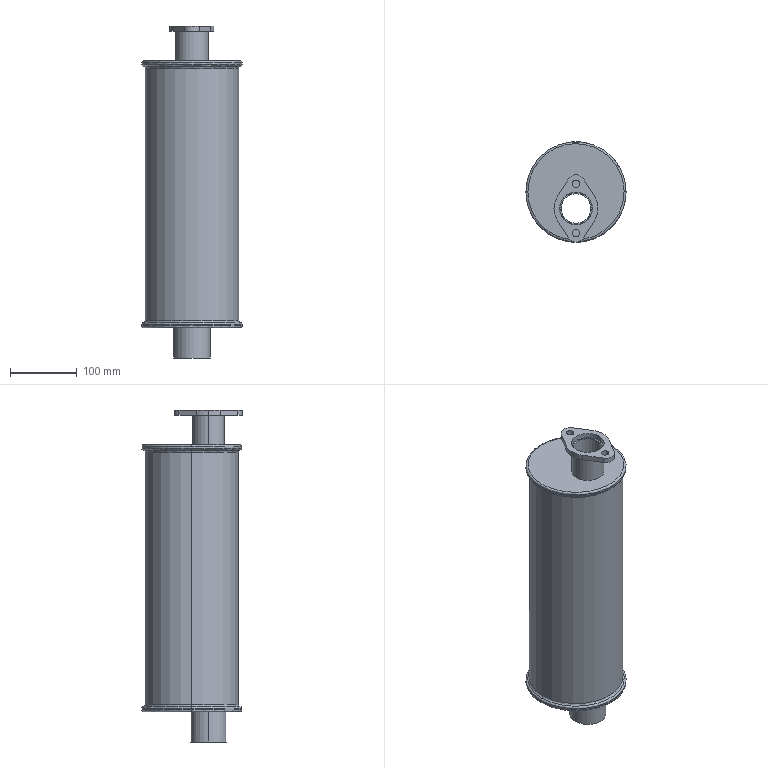Part | SolidWorks | features BaseBody 2 | 2 solids | 51 faces | box 150 x 150.5 x 497 mm | volume 633122 mm3 | cylinder 27 | plane 12 | spline 12 | commonest cylinder face diameters 11 x4 150 x4 66 x3 27 x2 44 x2 48 x2